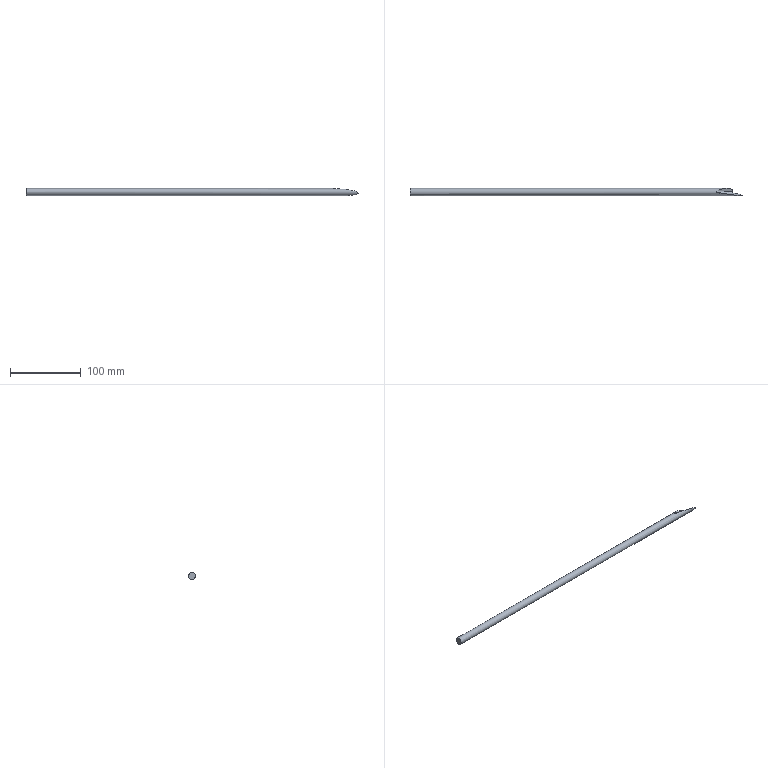Part | STEP file | solid 191 | 1 solid | 5 faces | box 469.808 x 10.006 x 10.001 mm | volume 35280 mm3 | spline 3 | cylinder 1 | plane 1 | commonest cylinder face diameters 10 x1